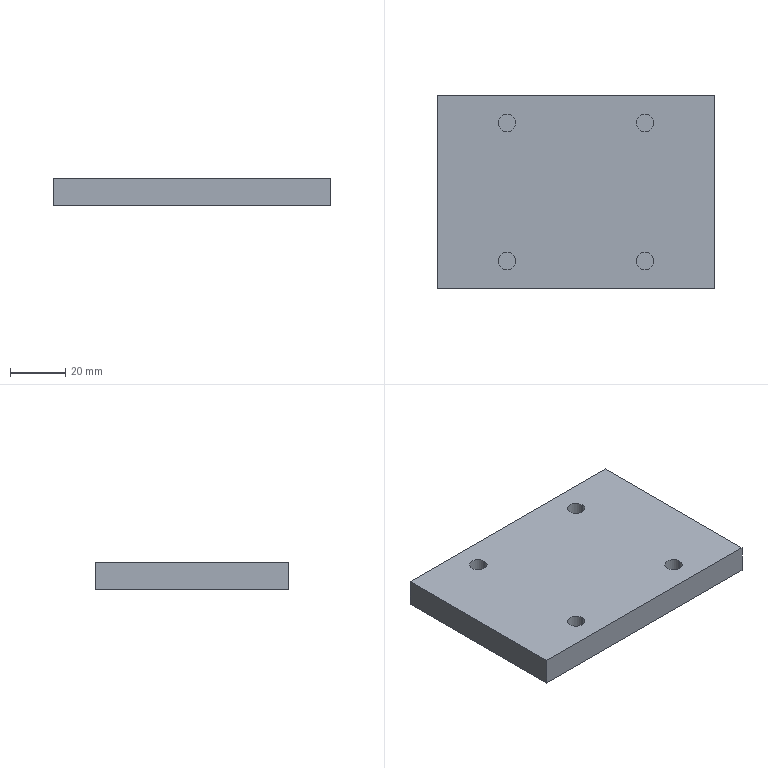Part | SolidWorks | features BaseBody 1 | 1 solid | 18 faces | box 100 x 70 x 10 mm | volume 68978 mm3 | plane 10 | cylinder 8 | commonest cylinder face diameters 6.3 x8
STEP:
#1=CARTESIAN_POINT('',(21.85,25.,-3.2));
#2=VERTEX_POINT('',#1);
#3=CARTESIAN_POINT('',(28.15,25.,-3.2));
#4=VERTEX_POINT('',#3);
#5=CARTESIAN_POINT('',(25.,25.,-3.2));
#6=DIRECTION('',(0.,0.,1.));
#7=DIRECTION('',(1.,0.,0.));
#8=AXIS2_PLACEMENT_3D('',#5,#6,#7);
#9=CIRCLE('',#8,3.15);
#10=EDGE_CURVE('',#2,#4,#9,.T.);
#11=ORIENTED_EDGE('',*,*,#10,.F.);
#12=CARTESIAN_POINT('',(21.85,25.,5.));
#13=VERTEX_POINT('',#12);
#14=CARTESIAN_POINT('',(21.85,25.,-3.2));
#15=DIRECTION('',(0.,0.,1.));
#16=VECTOR('',#15,1000.);
#17=LINE('',#14,#16);
#18=EDGE_CURVE('',#2,#13,#17,.T.);
#19=ORIENTED_EDGE('',*,*,#18,.T.);
#20=CARTESIAN_POINT('',(28.15,25.,5.));
#21=VERTEX_POINT('',#20);
#22=CARTESIAN_POINT('',(25.,25.,5.));
#23=DIRECTION('',(0.,0.,-1.));
#24=DIRECTION('',(1.,0.,0.));
#25=AXIS2_PLACEMENT_3D('',#22,#23,#24);
#26=CIRCLE('',#25,3.15);
#27=EDGE_CURVE('',#21,#13,#26,.T.);
#28=ORIENTED_EDGE('',*,*,#27,.F.);
#29=CARTESIAN_POINT('',(28.15,25.,-3.2));
#30=DIRECTION('',(0.,0.,1.));
#31=VECTOR('',#30,1000.);
#32=LINE('',#29,#31);
#33=EDGE_CURVE('',#4,#21,#32,.T.);
#34=ORIENTED_EDGE('',*,*,#33,.F.);
#35=EDGE_LOOP('',(#11,#19,#28,#34));
#36=FACE_OUTER_BOUND('',#35,.T.);
#37=CARTESIAN_POINT('',(25.,25.,-3.2));
#38=DIRECTION('',(0.,0.,1.));
#39=DIRECTION('',(1.,0.,0.));
#40=AXIS2_PLACEMENT_3D('',#37,#38,#39);
#41=CYLINDRICAL_SURFACE('',#40,3.15);
#42=ADVANCED_FACE('',(#36),#41,.F.);
#43=CARTESIAN_POINT('',(-28.15,25.,-3.2));
#44=VERTEX_POINT('',#43);
#45=CARTESIAN_POINT('',(-21.85,25.,-3.2));
#46=VERTEX_POINT('',#45);
#47=CARTESIAN_POINT('',(-25.,25.,-3.2));
#48=DIRECTION('',(0.,0.,1.));
#49=DIRECTION('',(1.,0.,0.));
#50=AXIS2_PLACEMENT_3D('',#47,#48,#49);
#51=CIRCLE('',#50,3.15);
#52=EDGE_CURVE('',#44,#46,#51,.T.);
#53=ORIENTED_EDGE('',*,*,#52,.F.);
#54=CARTESIAN_POINT('',(-28.15,25.,5.));
#55=VERTEX_POINT('',#54);
#56=CARTESIAN_POINT('',(-28.15,25.,-3.2));
#57=DIRECTION('',(0.,0.,1.));
#58=VECTOR('',#57,1000.);
#59=LINE('',#56,#58);
#60=EDGE_CURVE('',#44,#55,#59,.T.);
#61=ORIENTED_EDGE('',*,*,#60,.T.);
#62=CARTESIAN_POINT('',(-21.85,25.,5.));
#63=VERTEX_POINT('',#62);
#64=CARTESIAN_POINT('',(-25.,25.,5.));
#65=DIRECTION('',(0.,0.,-1.));
#66=DIRECTION('',(1.,0.,0.));
#67=AXIS2_PLACEMENT_3D('',#64,#65,#66);
#68=CIRCLE('',#67,3.15);
#69=EDGE_CURVE('',#63,#55,#68,.T.);
#70=ORIENTED_EDGE('',*,*,#69,.F.);
#71=CARTESIAN_POINT('',(-21.85,25.,-3.2));
#72=DIRECTION('',(0.,0.,1.));
#73=VECTOR('',#72,1000.);
#74=LINE('',#71,#73);
#75=EDGE_CURVE('',#46,#63,#74,.T.);
#76=ORIENTED_EDGE('',*,*,#75,.F.);
#77=EDGE_LOOP('',(#53,#61,#70,#76));
#78=FACE_OUTER_BOUND('',#77,.T.);
#79=CARTESIAN_POINT('',(-25.,25.,-3.2));
#80=DIRECTION('',(0.,0.,1.));
#81=DIRECTION('',(1.,0.,0.));
#82=AXIS2_PLACEMENT_3D('',#79,#80,#81);
#83=CYLINDRICAL_SURFACE('',#82,3.15);
#84=ADVANCED_FACE('',(#78),#83,.F.);
#85=CARTESIAN_POINT('',(21.85,-25.,-3.2));
#86=VERTEX_POINT('',#85);
#87=CARTESIAN_POINT('',(28.15,-25.,-3.2));
#88=VERTEX_POINT('',#87);
#89=CARTESIAN_POINT('',(25.,-25.,-3.2));
#90=DIRECTION('',(0.,0.,1.));
#91=DIRECTION('',(1.,0.,0.));
#92=AXIS2_PLACEMENT_3D('',#89,#90,#91);
#93=CIRCLE('',#92,3.15);
#94=EDGE_CURVE('',#86,#88,#93,.T.);
#95=ORIENTED_EDGE('',*,*,#94,.F.);
#96=CARTESIAN_POINT('',(21.85,-25.,5.));
#97=VERTEX_POINT('',#96);
#98=CARTESIAN_POINT('',(21.85,-25.,-3.2));
#99=DIRECTION('',(0.,0.,1.));
#100=VECTOR('',#99,1000.);
#101=LINE('',#98,#100);
#102=EDGE_CURVE('',#86,#97,#101,.T.);
#103=ORIENTED_EDGE('',*,*,#102,.T.);
#104=CARTESIAN_POINT('',(28.15,-25.,5.));
#105=VERTEX_POINT('',#104);
#106=CARTESIAN_POINT('',(25.,-25.,5.));
#107=DIRECTION('',(0.,0.,-1.));
#108=DIRECTION('',(1.,0.,0.));
#109=AXIS2_PLACEMENT_3D('',#106,#107,#108);
#110=CIRCLE('',#109,3.15);
#111=EDGE_CURVE('',#105,#97,#110,.T.);
#112=ORIENTED_EDGE('',*,*,#111,.F.);
#113=CARTESIAN_POINT('',(28.15,-25.,-3.2));
#114=DIRECTION('',(0.,0.,1.));
#115=VECTOR('',#114,1000.);
#116=LINE('',#113,#115);
#117=EDGE_CURVE('',#88,#105,#116,.T.);
#118=ORIENTED_EDGE('',*,*,#117,.F.);
#119=EDGE_LOOP('',(#95,#103,#112,#118));
#120=FACE_OUTER_BOUND('',#119,.T.);
#121=CARTESIAN_POINT('',(25.,-25.,-3.2));
#122=DIRECTION('',(0.,0.,1.));
#123=DIRECTION('',(1.,0.,0.));
#124=AXIS2_PLACEMENT_3D('',#121,#122,#123);
#125=CYLINDRICAL_SURFACE('',#124,3.15);
#126=ADVANCED_FACE('',(#120),#125,.F.);
#127=CARTESIAN_POINT('',(-28.15,-25.,-3.2));
#128=VERTEX_POINT('',#127);
#129=CARTESIAN_POINT('',(-21.85,-25.,-3.2));
#130=VERTEX_POINT('',#129);
#131=CARTESIAN_POINT('',(-25.,-25.,-3.2));
#132=DIRECTION('',(0.,0.,1.));
#133=DIRECTION('',(1.,0.,0.));
#134=AXIS2_PLACEMENT_3D('',#131,#132,#133);
#135=CIRCLE('',#134,3.15);
#136=EDGE_CURVE('',#128,#130,#135,.T.);
#137=ORIENTED_EDGE('',*,*,#136,.F.);
#138=CARTESIAN_POINT('',(-28.15,-25.,5.));
#139=VERTEX_POINT('',#138);
#140=CARTESIAN_POINT('',(-28.15,-25.,-3.2));
#141=DIRECTION('',(0.,0.,1.));
#142=VECTOR('',#141,1000.);
#143=LINE('',#140,#142);
#144=EDGE_CURVE('',#128,#139,#143,.T.);
#145=ORIENTED_EDGE('',*,*,#144,.T.);
#146=CARTESIAN_POINT('',(-21.85,-25.,5.));
#147=VERTEX_POINT('',#146);
#148=CARTESIAN_POINT('',(-25.,-25.,5.));
#149=DIRECTION('',(0.,0.,-1.));
#150=DIRECTION('',(1.,0.,0.));
#151=AXIS2_PLACEMENT_3D('',#148,#149,#150);
#152=CIRCLE('',#151,3.15);
#153=EDGE_CURVE('',#147,#139,#152,.T.);
#154=ORIENTED_EDGE('',*,*,#153,.F.);
#155=CARTESIAN_POINT('',(-21.85,-25.,-3.2));
#156=DIRECTION('',(0.,0.,1.));
#157=VECTOR('',#156,1000.);
#158=LINE('',#155,#157);
#159=EDGE_CURVE('',#130,#147,#158,.T.);
#160=ORIENTED_EDGE('',*,*,#159,.F.);
#161=EDGE_LOOP('',(#137,#145,#154,#160));
#162=FACE_OUTER_BOUND('',#161,.T.);
#163=CARTESIAN_POINT('',(-25.,-25.,-3.2));
#164=DIRECTION('',(0.,0.,1.));
#165=DIRECTION('',(1.,0.,0.));
#166=AXIS2_PLACEMENT_3D('',#163,#164,#165);
#167=CYLINDRICAL_SURFACE('',#166,3.15);
#168=ADVANCED_FACE('',(#162),#167,.F.);
#169=CARTESIAN_POINT('',(50.,-35.,-5.));
#170=VERTEX_POINT('',#169);
#171=CARTESIAN_POINT('',(50.,35.,-5.));
#172=VERTEX_POINT('',#171);
#173=CARTESIAN_POINT('',(50.,-35.,-5.));
#174=DIRECTION('',(0.,1.,0.));
#175=VECTOR('',#174,1000.);
#176=LINE('',#173,#175);
#177=EDGE_CURVE('',#170,#172,#176,.T.);
#178=ORIENTED_EDGE('',*,*,#177,.F.);
#179=CARTESIAN_POINT('',(-50.,-35.,-5.));
#180=VERTEX_POINT('',#179);
#181=CARTESIAN_POINT('',(-50.,-35.,-5.));
#182=DIRECTION('',(1.,0.,0.));
#183=VECTOR('',#182,1000.);
#184=LINE('',#181,#183);
#185=EDGE_CURVE('',#180,#170,#184,.T.);
#186=ORIENTED_EDGE('',*,*,#185,.F.);
#187=CARTESIAN_POINT('',(-50.,35.,-5.));
#188=VERTEX_POINT('',#187);
#189=CARTESIAN_POINT('',(-50.,-35.,-5.));
#190=DIRECTION('',(0.,-1.,0.));
#191=VECTOR('',#190,1000.);
#192=LINE('',#189,#191);
#193=EDGE_CURVE('',#188,#180,#192,.T.);
#194=ORIENTED_EDGE('',*,*,#193,.F.);
#195=CARTESIAN_POINT('',(-50.,35.,-5.));
#196=DIRECTION('',(-1.,0.,0.));
#197=VECTOR('',#196,1000.);
#198=LINE('',#195,#197);
#199=EDGE_CURVE('',#172,#188,#198,.T.);
#200=ORIENTED_EDGE('',*,*,#199,.F.);
#201=EDGE_LOOP('',(#178,#186,#194,#200));
#202=FACE_OUTER_BOUND('',#201,.T.);
#203=CARTESIAN_POINT('',(-50.,-35.,-5.));
#204=DIRECTION('',(0.,0.,1.));
#205=DIRECTION('',(1.,0.,0.));
#206=AXIS2_PLACEMENT_3D('',#203,#204,#205);
#207=PLANE('',#206);
#208=ADVANCED_FACE('',(#202),#207,.F.);
#209=CARTESIAN_POINT('',(-50.,35.,5.));
#210=VERTEX_POINT('',#209);
#211=CARTESIAN_POINT('',(50.,35.,5.));
#212=VERTEX_POINT('',#211);
#213=CARTESIAN_POINT('',(-50.,35.,5.));
#214=DIRECTION('',(1.,0.,0.));
#215=VECTOR('',#214,1000.);
#216=LINE('',#213,#215);
#217=EDGE_CURVE('',#210,#212,#216,.T.);
#218=ORIENTED_EDGE('',*,*,#217,.T.);
#219=CARTESIAN_POINT('',(50.,35.,-5.));
#220=DIRECTION('',(0.,0.,-1.));
#221=VECTOR('',#220,1000.);
#222=LINE('',#219,#221);
#223=EDGE_CURVE('',#212,#172,#222,.T.);
#224=ORIENTED_EDGE('',*,*,#223,.T.);
#225=ORIENTED_EDGE('',*,*,#199,.T.);
#226=CARTESIAN_POINT('',(-50.,35.,-5.));
#227=DIRECTION('',(0.,0.,1.));
#228=VECTOR('',#227,1000.);
#229=LINE('',#226,#228);
#230=EDGE_CURVE('',#188,#210,#229,.T.);
#231=ORIENTED_EDGE('',*,*,#230,.T.);
#232=EDGE_LOOP('',(#218,#224,#225,#231));
#233=FACE_OUTER_BOUND('',#232,.T.);
#234=CARTESIAN_POINT('',(-50.,35.,-5.));
#235=DIRECTION('',(0.,1.,0.));
#236=DIRECTION('',(0.,0.,1.));
#237=AXIS2_PLACEMENT_3D('',#234,#235,#236);
#238=PLANE('',#237);
#239=ADVANCED_FACE('',(#233),#238,.T.);
#240=ORIENTED_EDGE('',*,*,#223,.F.);
#241=CARTESIAN_POINT('',(50.,-35.,5.));
#242=VERTEX_POINT('',#241);
#243=CARTESIAN_POINT('',(50.,-35.,5.));
#244=DIRECTION('',(0.,-1.,0.));
#245=VECTOR('',#244,1000.);
#246=LINE('',#243,#245);
#247=EDGE_CURVE('',#212,#242,#246,.T.);
#248=ORIENTED_EDGE('',*,*,#247,.T.);
#249=CARTESIAN_POINT('',(50.,-35.,-5.));
#250=DIRECTION('',(0.,0.,-1.));
#251=VECTOR('',#250,1000.);
#252=LINE('',#249,#251);
#253=EDGE_CURVE('',#242,#170,#252,.T.);
#254=ORIENTED_EDGE('',*,*,#253,.T.);
#255=ORIENTED_EDGE('',*,*,#177,.T.);
#256=EDGE_LOOP('',(#240,#248,#254,#255));
#257=FACE_OUTER_BOUND('',#256,.T.);
#258=CARTESIAN_POINT('',(50.,-35.,-5.));
#259=DIRECTION('',(1.,0.,0.));
#260=DIRECTION('',(0.,0.,-1.));
#261=AXIS2_PLACEMENT_3D('',#258,#259,#260);
#262=PLANE('',#261);
#263=ADVANCED_FACE('',(#257),#262,.T.);
#264=CARTESIAN_POINT('',(-50.,-35.,5.));
#265=VERTEX_POINT('',#264);
#266=CARTESIAN_POINT('',(-50.,-35.,5.));
#267=DIRECTION('',(1.,0.,0.));
#268=VECTOR('',#267,1000.);
#269=LINE('',#266,#268);
#270=EDGE_CURVE('',#265,#242,#269,.T.);
#271=ORIENTED_EDGE('',*,*,#270,.F.);
#272=CARTESIAN_POINT('',(-50.,-35.,-5.));
#273=DIRECTION('',(0.,0.,1.));
#274=VECTOR('',#273,1000.);
#275=LINE('',#272,#274);
#276=EDGE_CURVE('',#180,#265,#275,.T.);
#277=ORIENTED_EDGE('',*,*,#276,.F.);
#278=ORIENTED_EDGE('',*,*,#185,.T.);
#279=ORIENTED_EDGE('',*,*,#253,.F.);
#280=EDGE_LOOP('',(#271,#277,#278,#279));
#281=FACE_OUTER_BOUND('',#280,.T.);
#282=CARTESIAN_POINT('',(-50.,-35.,-5.));
#283=DIRECTION('',(0.,1.,0.));
#284=DIRECTION('',(0.,0.,1.));
#285=AXIS2_PLACEMENT_3D('',#282,#283,#284);
#286=PLANE('',#285);
#287=ADVANCED_FACE('',(#281),#286,.F.);
#288=ORIENTED_EDGE('',*,*,#230,.F.);
#289=ORIENTED_EDGE('',*,*,#193,.T.);
#290=ORIENTED_EDGE('',*,*,#276,.T.);
#291=CARTESIAN_POINT('',(-50.,-35.,5.));
#292=DIRECTION('',(0.,-1.,0.));
#293=VECTOR('',#292,1000.);
#294=LINE('',#291,#293);
#295=EDGE_CURVE('',#210,#265,#294,.T.);
#296=ORIENTED_EDGE('',*,*,#295,.F.);
#297=EDGE_LOOP('',(#288,#289,#290,#296));
#298=FACE_OUTER_BOUND('',#297,.T.);
#299=CARTESIAN_POINT('',(-50.,-35.,-5.));
#300=DIRECTION('',(1.,0.,0.));
#301=DIRECTION('',(0.,0.,-1.));
#302=AXIS2_PLACEMENT_3D('',#299,#300,#301);
#303=PLANE('',#302);
#304=ADVANCED_FACE('',(#298),#303,.F.);
#305=ORIENTED_EDGE('',*,*,#27,.T.);
#306=CARTESIAN_POINT('',(25.,25.,5.));
#307=DIRECTION('',(0.,0.,-1.));
#308=DIRECTION('',(1.,0.,0.));
#309=AXIS2_PLACEMENT_3D('',#306,#307,#308);
#310=CIRCLE('',#309,3.15);
#311=EDGE_CURVE('',#13,#21,#310,.T.);
#312=ORIENTED_EDGE('',*,*,#311,.T.);
#313=EDGE_LOOP('',(#305,#312));
#314=FACE_BOUND('',#313,.T.);
#315=ORIENTED_EDGE('',*,*,#69,.T.);
#316=CARTESIAN_POINT('',(-25.,25.,5.));
#317=DIRECTION('',(0.,0.,-1.));
#318=DIRECTION('',(1.,0.,0.));
#319=AXIS2_PLACEMENT_3D('',#316,#317,#318);
#320=CIRCLE('',#319,3.15);
#321=EDGE_CURVE('',#55,#63,#320,.T.);
#322=ORIENTED_EDGE('',*,*,#321,.T.);
#323=EDGE_LOOP('',(#315,#322));
#324=FACE_BOUND('',#323,.T.);
#325=ORIENTED_EDGE('',*,*,#111,.T.);
#326=CARTESIAN_POINT('',(25.,-25.,5.));
#327=DIRECTION('',(0.,0.,-1.));
#328=DIRECTION('',(1.,0.,0.));
#329=AXIS2_PLACEMENT_3D('',#326,#327,#328);
#330=CIRCLE('',#329,3.15);
#331=EDGE_CURVE('',#97,#105,#330,.T.);
#332=ORIENTED_EDGE('',*,*,#331,.T.);
#333=EDGE_LOOP('',(#325,#332));
#334=FACE_BOUND('',#333,.T.);
#335=ORIENTED_EDGE('',*,*,#153,.T.);
#336=CARTESIAN_POINT('',(-25.,-25.,5.));
#337=DIRECTION('',(0.,0.,-1.));
#338=DIRECTION('',(1.,0.,0.));
#339=AXIS2_PLACEMENT_3D('',#336,#337,#338);
#340=CIRCLE('',#339,3.15);
#341=EDGE_CURVE('',#139,#147,#340,.T.);
#342=ORIENTED_EDGE('',*,*,#341,.T.);
#343=EDGE_LOOP('',(#335,#342));
#344=FACE_BOUND('',#343,.T.);
#345=ORIENTED_EDGE('',*,*,#247,.F.);
#346=ORIENTED_EDGE('',*,*,#217,.F.);
#347=ORIENTED_EDGE('',*,*,#295,.T.);
#348=ORIENTED_EDGE('',*,*,#270,.T.);
#349=EDGE_LOOP('',(#345,#346,#347,#348));
#350=FACE_OUTER_BOUND('',#349,.T.);
#351=CARTESIAN_POINT('',(-50.,-35.,5.));
#352=DIRECTION('',(0.,0.,1.));
#353=DIRECTION('',(1.,0.,0.));
#354=AXIS2_PLACEMENT_3D('',#351,#352,#353);
#355=PLANE('',#354);
#356=ADVANCED_FACE('',(#314,#324,#334,#344,#350),#355,.T.);
#357=ORIENTED_EDGE('',*,*,#18,.F.);
#358=CARTESIAN_POINT('',(25.,25.,-3.2));
#359=DIRECTION('',(0.,0.,1.));
#360=DIRECTION('',(1.,0.,0.));
#361=AXIS2_PLACEMENT_3D('',#358,#359,#360);
#362=CIRCLE('',#361,3.15);
#363=EDGE_CURVE('',#4,#2,#362,.T.);
#364=ORIENTED_EDGE('',*,*,#363,.F.);
#365=ORIENTED_EDGE('',*,*,#33,.T.);
#366=ORIENTED_EDGE('',*,*,#311,.F.);
#367=EDGE_LOOP('',(#357,#364,#365,#366));
#368=FACE_OUTER_BOUND('',#367,.T.);
#369=CARTESIAN_POINT('',(25.,25.,-3.2));
#370=DIRECTION('',(0.,0.,1.));
#371=DIRECTION('',(1.,0.,0.));
#372=AXIS2_PLACEMENT_3D('',#369,#370,#371);
#373=CYLINDRICAL_SURFACE('',#372,3.15);
#374=ADVANCED_FACE('',(#368),#373,.F.);
#375=ORIENTED_EDGE('',*,*,#60,.F.);
#376=CARTESIAN_POINT('',(-25.,25.,-3.2));
#377=DIRECTION('',(0.,0.,1.));
#378=DIRECTION('',(1.,0.,0.));
#379=AXIS2_PLACEMENT_3D('',#376,#377,#378);
#380=CIRCLE('',#379,3.15);
#381=EDGE_CURVE('',#46,#44,#380,.T.);
#382=ORIENTED_EDGE('',*,*,#381,.F.);
#383=ORIENTED_EDGE('',*,*,#75,.T.);
#384=ORIENTED_EDGE('',*,*,#321,.F.);
#385=EDGE_LOOP('',(#375,#382,#383,#384));
#386=FACE_OUTER_BOUND('',#385,.T.);
#387=CARTESIAN_POINT('',(-25.,25.,-3.2));
#388=DIRECTION('',(0.,0.,1.));
#389=DIRECTION('',(1.,0.,0.));
#390=AXIS2_PLACEMENT_3D('',#387,#388,#389);
#391=CYLINDRICAL_SURFACE('',#390,3.15);
#392=ADVANCED_FACE('',(#386),#391,.F.);
#393=ORIENTED_EDGE('',*,*,#102,.F.);
#394=CARTESIAN_POINT('',(25.,-25.,-3.2));
#395=DIRECTION('',(0.,0.,1.));
#396=DIRECTION('',(1.,0.,0.));
#397=AXIS2_PLACEMENT_3D('',#394,#395,#396);
#398=CIRCLE('',#397,3.15);
#399=EDGE_CURVE('',#88,#86,#398,.T.);
#400=ORIENTED_EDGE('',*,*,#399,.F.);
#401=ORIENTED_EDGE('',*,*,#117,.T.);
#402=ORIENTED_EDGE('',*,*,#331,.F.);
#403=EDGE_LOOP('',(#393,#400,#401,#402));
#404=FACE_OUTER_BOUND('',#403,.T.);
#405=CARTESIAN_POINT('',(25.,-25.,-3.2));
#406=DIRECTION('',(0.,0.,1.));
#407=DIRECTION('',(1.,0.,0.));
#408=AXIS2_PLACEMENT_3D('',#405,#406,#407);
#409=CYLINDRICAL_SURFACE('',#408,3.15);
#410=ADVANCED_FACE('',(#404),#409,.F.);
#411=ORIENTED_EDGE('',*,*,#144,.F.);
#412=CARTESIAN_POINT('',(-25.,-25.,-3.2));
#413=DIRECTION('',(0.,0.,1.));
#414=DIRECTION('',(1.,0.,0.));
#415=AXIS2_PLACEMENT_3D('',#412,#413,#414);
#416=CIRCLE('',#415,3.15);
#417=EDGE_CURVE('',#130,#128,#416,.T.);
#418=ORIENTED_EDGE('',*,*,#417,.F.);
#419=ORIENTED_EDGE('',*,*,#159,.T.);
#420=ORIENTED_EDGE('',*,*,#341,.F.);
#421=EDGE_LOOP('',(#411,#418,#419,#420));
#422=FACE_OUTER_BOUND('',#421,.T.);
#423=CARTESIAN_POINT('',(-25.,-25.,-3.2));
#424=DIRECTION('',(0.,0.,1.));
#425=DIRECTION('',(1.,0.,0.));
#426=AXIS2_PLACEMENT_3D('',#423,#424,#425);
#427=CYLINDRICAL_SURFACE('',#426,3.15);
#428=ADVANCED_FACE('',(#422),#427,.F.);
#429=ORIENTED_EDGE('',*,*,#363,.T.);
#430=ORIENTED_EDGE('',*,*,#10,.T.);
#431=EDGE_LOOP('',(#429,#430));
#432=FACE_OUTER_BOUND('',#431,.T.);
#433=CARTESIAN_POINT('',(25.,25.,-3.2));
#434=DIRECTION('',(0.,0.,1.));
#435=DIRECTION('',(1.,0.,0.));
#436=AXIS2_PLACEMENT_3D('',#433,#434,#435);
#437=PLANE('',#436);
#438=ADVANCED_FACE('',(#432),#437,.T.);
#439=ORIENTED_EDGE('',*,*,#381,.T.);
#440=ORIENTED_EDGE('',*,*,#52,.T.);
#441=EDGE_LOOP('',(#439,#440));
#442=FACE_OUTER_BOUND('',#441,.T.);
#443=CARTESIAN_POINT('',(-25.,25.,-3.2));
#444=DIRECTION('',(0.,0.,1.));
#445=DIRECTION('',(1.,0.,0.));
#446=AXIS2_PLACEMENT_3D('',#443,#444,#445);
#447=PLANE('',#446);
#448=ADVANCED_FACE('',(#442),#447,.T.);
#449=ORIENTED_EDGE('',*,*,#399,.T.);
#450=ORIENTED_EDGE('',*,*,#94,.T.);
#451=EDGE_LOOP('',(#449,#450));
#452=FACE_OUTER_BOUND('',#451,.T.);
#453=CARTESIAN_POINT('',(25.,-25.,-3.2));
#454=DIRECTION('',(0.,0.,1.));
#455=DIRECTION('',(1.,0.,0.));
#456=AXIS2_PLACEMENT_3D('',#453,#454,#455);
#457=PLANE('',#456);
#458=ADVANCED_FACE('',(#452),#457,.T.);
#459=ORIENTED_EDGE('',*,*,#417,.T.);
#460=ORIENTED_EDGE('',*,*,#136,.T.);
#461=EDGE_LOOP('',(#459,#460));
#462=FACE_OUTER_BOUND('',#461,.T.);
#463=CARTESIAN_POINT('',(-25.,-25.,-3.2));
#464=DIRECTION('',(0.,0.,1.));
#465=DIRECTION('',(1.,0.,0.));
#466=AXIS2_PLACEMENT_3D('',#463,#464,#465);
#467=PLANE('',#466);
#468=ADVANCED_FACE('',(#462),#467,.T.);
#469=CLOSED_SHELL('',(#42,#84,#126,#168,#208,#239,#263,#287,#304,#356,#374,#392,#410,#428,#438,#448,#458,#468));
#470=MANIFOLD_SOLID_BREP('',#469);
#471=CARTESIAN_POINT('',(0.,0.,0.));
#472=DIRECTION('',(0.,0.,1.));
#473=DIRECTION('',(1.,0.,0.));
#474=AXIS2_PLACEMENT_3D('',#471,#472,#473);
#475=(LENGTH_UNIT()NAMED_UNIT(*)SI_UNIT(.MILLI.,.METRE.));
#476=UNCERTAINTY_MEASURE_WITH_UNIT(LENGTH_MEASURE(0.00001),#475,'','');
#477=(NAMED_UNIT(*)PLANE_ANGLE_UNIT()SI_UNIT($,.RADIAN.));
#478=(NAMED_UNIT(*)SI_UNIT($,.STERADIAN.)SOLID_ANGLE_UNIT());
#479=(GEOMETRIC_REPRESENTATION_CONTEXT(3)GLOBAL_UNCERTAINTY_ASSIGNED_CONTEXT((#476))GLOBAL_UNIT_ASSIGNED_CONTEXT((#475,#477,#478))REPRESENTATION_CONTEXT('',''));
#480=ADVANCED_BREP_SHAPE_REPRESENTATION('',(#470,#474),#479);